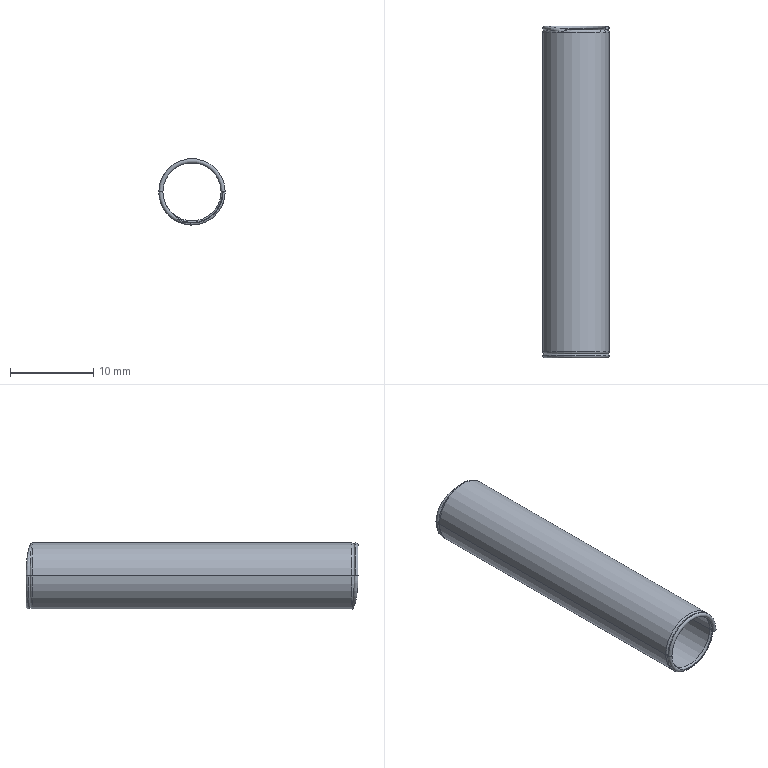Part | NX | 1 solid | 26 faces | box 8 x 40 x 8 mm | volume 464.179 mm3 | torus 18 | plane 4 | cylinder 4 | commonest cylinder face diameters 7 x2 8 x2
STEP:
#1=CARTESIAN_POINT('',(-3.75,19.5,0.));
#2=VERTEX_POINT('',#1);
#3=CARTESIAN_POINT('',(3.75,19.5,0.));
#4=VERTEX_POINT('',#3);
#5=CARTESIAN_POINT('',(0.,19.5,0.));
#6=DIRECTION('',(0.,1.,0.));
#7=DIRECTION('',(1.,0.,0.));
#8=AXIS2_PLACEMENT_3D('',#5,#6,#7);
#9=CIRCLE('',#8,3.75);
#10=EDGE_CURVE('',#2,#4,#9,.T.);
#11=ORIENTED_EDGE('',*,*,#10,.F.);
#12=CARTESIAN_POINT('',(-3.5,19.75,0.));
#13=VERTEX_POINT('',#12);
#14=CARTESIAN_POINT('',(-3.75,19.75,0.));
#15=DIRECTION('',(0.,0.,-1.));
#16=DIRECTION('',(-1.,0.,0.));
#17=AXIS2_PLACEMENT_3D('',#14,#15,#16);
#18=CIRCLE('',#17,0.25);
#19=EDGE_CURVE('',#13,#2,#18,.T.);
#20=ORIENTED_EDGE('',*,*,#19,.F.);
#21=CARTESIAN_POINT('',(-3.5,19.75,0.0215));
#22=VERTEX_POINT('',#21);
#23=CARTESIAN_POINT('',(0.,19.75,0.));
#24=DIRECTION('',(0.,-1.,0.));
#25=DIRECTION('',(-1.,0.,0.));
#26=AXIS2_PLACEMENT_3D('',#23,#24,#25);
#27=CIRCLE('',#26,3.5);
#28=EDGE_CURVE('',#22,#13,#27,.T.);
#29=ORIENTED_EDGE('',*,*,#28,.F.);
#30=CARTESIAN_POINT('',(-0.9578,19.51,3.553));
#31=VERTEX_POINT('',#30);
#32=CARTESIAN_POINT('',(-3.5,19.75,0.0215));
#33=CARTESIAN_POINT('',(-3.497,19.75,0.5366));
#34=CARTESIAN_POINT('',(-3.313,19.735,1.301));
#35=CARTESIAN_POINT('',(-2.804,19.689,2.155));
#36=CARTESIAN_POINT('',(-2.079,19.621,2.924));
#37=CARTESIAN_POINT('',(-1.377,19.557,3.326));
#38=CARTESIAN_POINT('',(-1.039,19.52,3.495));
#39=CARTESIAN_POINT('',(-0.9578,19.51,3.553));
#40=B_SPLINE_CURVE_WITH_KNOTS('',3,(#32,#33,#34,#35,#36,#37,#38,#39),.UNSPECIFIED.,.F.,.F.,(4,1,1,1,1,4),(0.,0.25,0.375,0.5,0.75,1.),.UNSPECIFIED.);
#41=EDGE_CURVE('',#31,#22,#40,.F.);
#42=ORIENTED_EDGE('',*,*,#41,.F.);
#43=CARTESIAN_POINT('',(3.68,19.51,0.));
#44=VERTEX_POINT('',#43);
#45=CARTESIAN_POINT('',(0.,19.51,0.));
#46=DIRECTION('',(0.,-1.,0.));
#47=DIRECTION('',(0.,0.,1.));
#48=AXIS2_PLACEMENT_3D('',#45,#46,#47);
#49=CIRCLE('',#48,3.68);
#50=EDGE_CURVE('',#44,#31,#49,.T.);
#51=ORIENTED_EDGE('',*,*,#50,.F.);
#52=CARTESIAN_POINT('',(3.75,19.75,0.));
#53=DIRECTION('',(0.,0.,1.));
#54=DIRECTION('',(1.,0.,0.));
#55=AXIS2_PLACEMENT_3D('',#52,#53,#54);
#56=CIRCLE('',#55,0.25);
#57=EDGE_CURVE('',#44,#4,#56,.T.);
#58=ORIENTED_EDGE('',*,*,#57,.T.);
#59=EDGE_LOOP('',(#11,#20,#29,#42,#51,#58));
#60=FACE_BOUND('',#59,.T.);
#61=CARTESIAN_POINT('',(0.,19.75,0.));
#62=DIRECTION('',(0.,-1.,0.));
#63=DIRECTION('',(-1.,0.,0.));
#64=AXIS2_PLACEMENT_3D('',#61,#62,#63);
#65=TOROIDAL_SURFACE('',#64,3.75,0.25);
#66=ADVANCED_FACE('',(#60),#65,.T.);
#67=ORIENTED_EDGE('',*,*,#50,.T.);
#68=CARTESIAN_POINT('',(-0.9704,19.51,3.622));
#69=VERTEX_POINT('',#68);
#70=CARTESIAN_POINT('',(-0.9578,19.51,3.553));
#71=CARTESIAN_POINT('',(-0.9429,19.51,3.581));
#72=CARTESIAN_POINT('',(-0.9471,19.51,3.604));
#73=CARTESIAN_POINT('',(-0.9704,19.51,3.622));
#74=B_SPLINE_CURVE_WITH_KNOTS('',3,(#70,#71,#72,#73),.UNSPECIFIED.,.F.,.F.,(4,4),(0.,1.),.UNSPECIFIED.);
#75=EDGE_CURVE('',#31,#69,#74,.T.);
#76=ORIENTED_EDGE('',*,*,#75,.T.);
#77=CARTESIAN_POINT('',(3.75,19.51,0.));
#78=VERTEX_POINT('',#77);
#79=CARTESIAN_POINT('',(0.,19.51,0.));
#80=DIRECTION('',(0.,1.,0.));
#81=DIRECTION('',(1.,0.,0.));
#82=AXIS2_PLACEMENT_3D('',#79,#80,#81);
#83=CIRCLE('',#82,3.75);
#84=EDGE_CURVE('',#69,#78,#83,.T.);
#85=ORIENTED_EDGE('',*,*,#84,.T.);
#86=CARTESIAN_POINT('',(2.812,19.51,0.));
#87=DIRECTION('',(-1.,0.,0.));
#88=VECTOR('',#87,1000.);
#89=LINE('',#86,#88);
#90=EDGE_CURVE('',#78,#44,#89,.T.);
#91=ORIENTED_EDGE('',*,*,#90,.T.);
#92=EDGE_LOOP('',(#67,#76,#85,#91));
#93=FACE_BOUND('',#92,.T.);
#94=CARTESIAN_POINT('',(1.875,19.51,0.));
#95=DIRECTION('',(0.,1.,0.));
#96=DIRECTION('',(1.,0.,0.));
#97=AXIS2_PLACEMENT_3D('',#94,#95,#96);
#98=PLANE('',#97);
#99=ADVANCED_FACE('',(#93),#98,.T.);
#100=CARTESIAN_POINT('',(-3.8,19.505,0.));
#101=VERTEX_POINT('',#100);
#102=CARTESIAN_POINT('',(-3.8,19.505,0.));
#103=CARTESIAN_POINT('',(-3.8,19.505,0.1204));
#104=CARTESIAN_POINT('',(-3.797,19.504,0.403));
#105=CARTESIAN_POINT('',(-3.736,19.496,0.9057));
#106=CARTESIAN_POINT('',(-3.632,19.485,1.311));
#107=CARTESIAN_POINT('',(-3.541,19.476,1.594));
#108=CARTESIAN_POINT('',(-3.335,19.457,2.05));
#109=CARTESIAN_POINT('',(-3.191,19.444,2.281));
#110=CARTESIAN_POINT('',(-2.929,19.422,2.652));
#111=CARTESIAN_POINT('',(-2.656,19.398,2.962));
#112=CARTESIAN_POINT('',(-2.045,19.364,3.43));
#113=CARTESIAN_POINT('',(-1.779,19.341,3.572));
#114=CARTESIAN_POINT('',(-1.267,19.4,3.777));
#115=CARTESIAN_POINT('',(-1.078,19.49,3.698));
#116=CARTESIAN_POINT('',(-1.043,19.51,3.679));
#117=CARTESIAN_POINT('',(-0.9704,19.51,3.622));
#118=B_SPLINE_CURVE_WITH_KNOTS('',3,(#102,#103,#104,#105,#106,#107,#108,#109,#110,#111,#112,#113,#114,#115,#116,#117),.UNSPECIFIED.,.F.,.F.,(4,1,1,1,1,1,1,1,1,1,1,1,1,4),(0.,0.0625,0.125,0.1562,0.1875,0.25,0.3125,0.375,0.5,0.625,0.75,0.875,0.9375,1.),.UNSPECIFIED.);
#119=EDGE_CURVE('',#69,#101,#118,.F.);
#120=ORIENTED_EDGE('',*,*,#119,.F.);
#121=ORIENTED_EDGE('',*,*,#75,.F.);
#122=ORIENTED_EDGE('',*,*,#41,.T.);
#123=ORIENTED_EDGE('',*,*,#28,.T.);
#124=CARTESIAN_POINT('',(-4.,19.75,0.));
#125=VERTEX_POINT('',#124);
#126=CARTESIAN_POINT('',(-3.75,19.75,0.));
#127=DIRECTION('',(0.,0.,-1.));
#128=DIRECTION('',(-1.,0.,0.));
#129=AXIS2_PLACEMENT_3D('',#126,#127,#128);
#130=CIRCLE('',#129,0.25);
#131=EDGE_CURVE('',#125,#13,#130,.T.);
#132=ORIENTED_EDGE('',*,*,#131,.F.);
#133=CARTESIAN_POINT('',(-3.75,19.75,0.));
#134=DIRECTION('',(0.,0.,-1.));
#135=DIRECTION('',(-1.,0.,0.));
#136=AXIS2_PLACEMENT_3D('',#133,#134,#135);
#137=CIRCLE('',#136,0.25);
#138=EDGE_CURVE('',#101,#125,#137,.T.);
#139=ORIENTED_EDGE('',*,*,#138,.F.);
#140=EDGE_LOOP('',(#120,#121,#122,#123,#132,#139));
#141=FACE_BOUND('',#140,.T.);
#142=CARTESIAN_POINT('',(-0.1131,19.109,0.));
#143=DIRECTION('',(-0.1736,-0.9848,0.));
#144=DIRECTION('',(-0.9848,0.1736,0.));
#145=AXIS2_PLACEMENT_3D('',#142,#143,#144);
#146=TOROIDAL_SURFACE('',#145,3.693,0.25);
#147=ADVANCED_FACE('',(#141),#146,.T.);
#148=CARTESIAN_POINT('',(3.68,-19.51,0.));
#149=VERTEX_POINT('',#148);
#150=CARTESIAN_POINT('',(-0.9578,-19.51,-3.553));
#151=VERTEX_POINT('',#150);
#152=CARTESIAN_POINT('',(0.,-19.51,0.));
#153=DIRECTION('',(0.,1.,0.));
#154=DIRECTION('',(0.,0.,1.));
#155=AXIS2_PLACEMENT_3D('',#152,#153,#154);
#156=CIRCLE('',#155,3.68);
#157=EDGE_CURVE('',#149,#151,#156,.T.);
#158=ORIENTED_EDGE('',*,*,#157,.T.);
#159=CARTESIAN_POINT('',(-0.9704,-19.51,-3.622));
#160=VERTEX_POINT('',#159);
#161=CARTESIAN_POINT('',(-0.9578,-19.51,-3.553));
#162=CARTESIAN_POINT('',(-0.9429,-19.51,-3.581));
#163=CARTESIAN_POINT('',(-0.9471,-19.51,-3.604));
#164=CARTESIAN_POINT('',(-0.9704,-19.51,-3.622));
#165=B_SPLINE_CURVE_WITH_KNOTS('',3,(#161,#162,#163,#164),.UNSPECIFIED.,.F.,.F.,(4,4),(0.,1.),.UNSPECIFIED.);
#166=EDGE_CURVE('',#151,#160,#165,.T.);
#167=ORIENTED_EDGE('',*,*,#166,.T.);
#168=CARTESIAN_POINT('',(3.75,-19.51,0.));
#169=VERTEX_POINT('',#168);
#170=CARTESIAN_POINT('',(0.,-19.51,0.));
#171=DIRECTION('',(0.,1.,0.));
#172=DIRECTION('',(1.,0.,0.));
#173=AXIS2_PLACEMENT_3D('',#170,#171,#172);
#174=CIRCLE('',#173,3.75);
#175=EDGE_CURVE('',#169,#160,#174,.T.);
#176=ORIENTED_EDGE('',*,*,#175,.F.);
#177=CARTESIAN_POINT('',(2.812,-19.51,0.));
#178=DIRECTION('',(-1.,0.,0.));
#179=VECTOR('',#178,1000.);
#180=LINE('',#177,#179);
#181=EDGE_CURVE('',#169,#149,#180,.T.);
#182=ORIENTED_EDGE('',*,*,#181,.T.);
#183=EDGE_LOOP('',(#158,#167,#176,#182));
#184=FACE_BOUND('',#183,.T.);
#185=CARTESIAN_POINT('',(1.875,-19.51,0.));
#186=DIRECTION('',(0.,-1.,0.));
#187=DIRECTION('',(0.,0.,-1.));
#188=AXIS2_PLACEMENT_3D('',#185,#186,#187);
#189=PLANE('',#188);
#190=ADVANCED_FACE('',(#184),#189,.T.);
#191=ORIENTED_EDGE('',*,*,#10,.T.);
#192=CARTESIAN_POINT('',(3.5,19.25,0.));
#193=VERTEX_POINT('',#192);
#194=CARTESIAN_POINT('',(3.75,19.25,0.));
#195=DIRECTION('',(0.,0.,-1.));
#196=DIRECTION('',(-1.,0.,0.));
#197=AXIS2_PLACEMENT_3D('',#194,#195,#196);
#198=CIRCLE('',#197,0.25);
#199=EDGE_CURVE('',#193,#4,#198,.T.);
#200=ORIENTED_EDGE('',*,*,#199,.F.);
#201=CARTESIAN_POINT('',(-3.5,19.25,0.));
#202=VERTEX_POINT('',#201);
#203=CARTESIAN_POINT('',(0.,19.25,0.));
#204=DIRECTION('',(0.,1.,0.));
#205=DIRECTION('',(1.,0.,0.));
#206=AXIS2_PLACEMENT_3D('',#203,#204,#205);
#207=CIRCLE('',#206,3.5);
#208=EDGE_CURVE('',#202,#193,#207,.T.);
#209=ORIENTED_EDGE('',*,*,#208,.F.);
#210=CARTESIAN_POINT('',(-3.75,19.25,0.));
#211=DIRECTION('',(0.,0.,1.));
#212=DIRECTION('',(1.,0.,0.));
#213=AXIS2_PLACEMENT_3D('',#210,#211,#212);
#214=CIRCLE('',#213,0.25);
#215=EDGE_CURVE('',#202,#2,#214,.T.);
#216=ORIENTED_EDGE('',*,*,#215,.T.);
#217=EDGE_LOOP('',(#191,#200,#209,#216));
#218=FACE_BOUND('',#217,.T.);
#219=CARTESIAN_POINT('',(0.,19.25,0.));
#220=DIRECTION('',(0.,1.,0.));
#221=DIRECTION('',(1.,0.,0.));
#222=AXIS2_PLACEMENT_3D('',#219,#220,#221);
#223=TOROIDAL_SURFACE('',#222,3.75,0.25);
#224=ADVANCED_FACE('',(#218),#223,.T.);
#225=CARTESIAN_POINT('',(-4.,-19.75,0.));
#226=VERTEX_POINT('',#225);
#227=CARTESIAN_POINT('',(-3.8,-19.505,0.));
#228=VERTEX_POINT('',#227);
#229=CARTESIAN_POINT('',(-3.75,-19.75,0.));
#230=DIRECTION('',(0.,0.,-1.));
#231=DIRECTION('',(-1.,0.,0.));
#232=AXIS2_PLACEMENT_3D('',#229,#230,#231);
#233=CIRCLE('',#232,0.25);
#234=EDGE_CURVE('',#226,#228,#233,.T.);
#235=ORIENTED_EDGE('',*,*,#234,.T.);
#236=CARTESIAN_POINT('',(-3.8,-19.505,0.));
#237=CARTESIAN_POINT('',(-3.8,-19.505,-0.1568));
#238=CARTESIAN_POINT('',(-3.794,-19.504,-0.4603));
#239=CARTESIAN_POINT('',(-3.721,-19.495,-0.9752));
#240=CARTESIAN_POINT('',(-3.549,-19.477,-1.621));
#241=CARTESIAN_POINT('',(-3.279,-19.452,-2.163));
#242=CARTESIAN_POINT('',(-2.911,-19.419,-2.695));
#243=CARTESIAN_POINT('',(-2.445,-19.384,-3.138));
#244=CARTESIAN_POINT('',(-2.135,-19.367,-3.356));
#245=CARTESIAN_POINT('',(-1.981,-19.359,-3.456));
#246=CARTESIAN_POINT('',(-1.669,-19.356,-3.619));
#247=CARTESIAN_POINT('',(-1.519,-19.361,-3.673));
#248=CARTESIAN_POINT('',(-1.282,-19.404,-3.765));
#249=CARTESIAN_POINT('',(-1.07,-19.492,-3.698));
#250=CARTESIAN_POINT('',(-1.042,-19.51,-3.678));
#251=CARTESIAN_POINT('',(-0.9704,-19.51,-3.622));
#252=B_SPLINE_CURVE_WITH_KNOTS('',3,(#236,#237,#238,#239,#240,#241,#242,#243,#244,#245,#246,#247,#248,#249,#250,#251),.UNSPECIFIED.,.F.,.F.,(4,1,1,1,1,1,1,1,1,1,1,1,1,4),(0.,0.125,0.1875,0.25,0.375,0.5,0.625,0.6875,0.75,0.8125,0.875,0.9375,0.9688,1.),.UNSPECIFIED.);
#253=EDGE_CURVE('',#160,#228,#252,.F.);
#254=ORIENTED_EDGE('',*,*,#253,.F.);
#255=ORIENTED_EDGE('',*,*,#166,.F.);
#256=CARTESIAN_POINT('',(-3.5,-19.75,-0.0215));
#257=VERTEX_POINT('',#256);
#258=CARTESIAN_POINT('',(-0.9578,-19.51,-3.553));
#259=CARTESIAN_POINT('',(-1.039,-19.52,-3.495));
#260=CARTESIAN_POINT('',(-1.302,-19.548,-3.374));
#261=CARTESIAN_POINT('',(-1.834,-19.599,-3.049));
#262=CARTESIAN_POINT('',(-2.247,-19.637,-2.744));
#263=CARTESIAN_POINT('',(-2.804,-19.687,-2.155));
#264=CARTESIAN_POINT('',(-3.311,-19.732,-1.305));
#265=CARTESIAN_POINT('',(-3.497,-19.75,-0.5384));
#266=CARTESIAN_POINT('',(-3.5,-19.75,-0.0215));
#267=B_SPLINE_CURVE_WITH_KNOTS('',3,(#258,#259,#260,#261,#262,#263,#264,#265,#266),.UNSPECIFIED.,.F.,.F.,(4,1,1,1,1,1,4),(0.,0.25,0.375,0.5,0.625,0.75,1.),.UNSPECIFIED.);
#268=EDGE_CURVE('',#257,#151,#267,.F.);
#269=ORIENTED_EDGE('',*,*,#268,.F.);
#270=CARTESIAN_POINT('',(-3.5,-19.75,0.));
#271=VERTEX_POINT('',#270);
#272=CARTESIAN_POINT('',(0.,-19.75,0.));
#273=DIRECTION('',(0.,-1.,0.));
#274=DIRECTION('',(-1.,0.,0.));
#275=AXIS2_PLACEMENT_3D('',#272,#273,#274);
#276=CIRCLE('',#275,3.5);
#277=EDGE_CURVE('',#257,#271,#276,.F.);
#278=ORIENTED_EDGE('',*,*,#277,.T.);
#279=CARTESIAN_POINT('',(-3.75,-19.75,0.));
#280=DIRECTION('',(0.,0.,-1.));
#281=DIRECTION('',(-1.,0.,0.));
#282=AXIS2_PLACEMENT_3D('',#279,#280,#281);
#283=CIRCLE('',#282,0.25);
#284=EDGE_CURVE('',#271,#226,#283,.T.);
#285=ORIENTED_EDGE('',*,*,#284,.T.);
#286=EDGE_LOOP('',(#235,#254,#255,#269,#278,#285));
#287=FACE_BOUND('',#286,.T.);
#288=CARTESIAN_POINT('',(-0.1131,-19.109,0.));
#289=DIRECTION('',(0.1736,-0.9848,0.));
#290=DIRECTION('',(-0.9848,-0.1736,0.));
#291=AXIS2_PLACEMENT_3D('',#288,#289,#290);
#292=TOROIDAL_SURFACE('',#291,3.693,0.25);
#293=ADVANCED_FACE('',(#287),#292,.T.);
#294=CARTESIAN_POINT('',(3.8,19.505,0.));
#295=VERTEX_POINT('',#294);
#296=CARTESIAN_POINT('',(3.75,19.26,0.));
#297=DIRECTION('',(0.,0.,-1.));
#298=DIRECTION('',(-1.,0.,0.));
#299=AXIS2_PLACEMENT_3D('',#296,#297,#298);
#300=CIRCLE('',#299,0.25);
#301=EDGE_CURVE('',#78,#295,#300,.T.);
#302=ORIENTED_EDGE('',*,*,#301,.T.);
#303=CARTESIAN_POINT('',(4.,19.75,0.));
#304=VERTEX_POINT('',#303);
#305=CARTESIAN_POINT('',(3.75,19.75,0.));
#306=DIRECTION('',(0.,0.,1.));
#307=DIRECTION('',(1.,0.,0.));
#308=AXIS2_PLACEMENT_3D('',#305,#306,#307);
#309=CIRCLE('',#308,0.25);
#310=EDGE_CURVE('',#295,#304,#309,.T.);
#311=ORIENTED_EDGE('',*,*,#310,.T.);
#312=CARTESIAN_POINT('',(3.5,19.75,0.));
#313=VERTEX_POINT('',#312);
#314=CARTESIAN_POINT('',(3.75,19.75,0.));
#315=DIRECTION('',(0.,0.,1.));
#316=DIRECTION('',(1.,0.,0.));
#317=AXIS2_PLACEMENT_3D('',#314,#315,#316);
#318=CIRCLE('',#317,0.25);
#319=EDGE_CURVE('',#304,#313,#318,.T.);
#320=ORIENTED_EDGE('',*,*,#319,.T.);
#321=CARTESIAN_POINT('',(3.75,19.75,0.));
#322=DIRECTION('',(0.,0.,1.));
#323=DIRECTION('',(1.,0.,0.));
#324=AXIS2_PLACEMENT_3D('',#321,#322,#323);
#325=CIRCLE('',#324,0.25);
#326=EDGE_CURVE('',#313,#44,#325,.T.);
#327=ORIENTED_EDGE('',*,*,#326,.T.);
#328=ORIENTED_EDGE('',*,*,#90,.F.);
#329=EDGE_LOOP('',(#302,#311,#320,#327,#328));
#330=FACE_BOUND('',#329,.T.);
#331=CARTESIAN_POINT('',(3.75,19.75,0.));
#332=DIRECTION('',(0.,0.,-1.));
#333=DIRECTION('',(-1.,0.,0.));
#334=AXIS2_PLACEMENT_3D('',#331,#332,#333);
#335=PLANE('',#334);
#336=ADVANCED_FACE('',(#330),#335,.F.);
#337=CARTESIAN_POINT('',(-3.75,-19.5,0.));
#338=VERTEX_POINT('',#337);
#339=CARTESIAN_POINT('',(3.75,-19.5,0.));
#340=VERTEX_POINT('',#339);
#341=CARTESIAN_POINT('',(0.,-19.5,0.));
#342=DIRECTION('',(0.,1.,0.));
#343=DIRECTION('',(1.,0.,0.));
#344=AXIS2_PLACEMENT_3D('',#341,#342,#343);
#345=CIRCLE('',#344,3.75);
#346=EDGE_CURVE('',#338,#340,#345,.T.);
#347=ORIENTED_EDGE('',*,*,#346,.T.);
#348=CARTESIAN_POINT('',(3.75,-19.75,0.));
#349=DIRECTION('',(0.,0.,1.));
#350=DIRECTION('',(1.,0.,0.));
#351=AXIS2_PLACEMENT_3D('',#348,#349,#350);
#352=CIRCLE('',#351,0.25);
#353=EDGE_CURVE('',#149,#340,#352,.F.);
#354=ORIENTED_EDGE('',*,*,#353,.F.);
#355=CARTESIAN_POINT('',(3.5,-19.75,0.));
#356=VERTEX_POINT('',#355);
#357=CARTESIAN_POINT('',(3.75,-19.75,0.));
#358=DIRECTION('',(0.,0.,1.));
#359=DIRECTION('',(1.,0.,0.));
#360=AXIS2_PLACEMENT_3D('',#357,#358,#359);
#361=CIRCLE('',#360,0.25);
#362=EDGE_CURVE('',#149,#356,#361,.T.);
#363=ORIENTED_EDGE('',*,*,#362,.T.);
#364=CARTESIAN_POINT('',(0.,-19.75,0.));
#365=DIRECTION('',(0.,-1.,0.));
#366=DIRECTION('',(-1.,0.,0.));
#367=AXIS2_PLACEMENT_3D('',#364,#365,#366);
#368=CIRCLE('',#367,3.5);
#369=EDGE_CURVE('',#356,#271,#368,.T.);
#370=ORIENTED_EDGE('',*,*,#369,.T.);
#371=CARTESIAN_POINT('',(-3.75,-19.75,0.));
#372=DIRECTION('',(0.,0.,-1.));
#373=DIRECTION('',(-1.,0.,0.));
#374=AXIS2_PLACEMENT_3D('',#371,#372,#373);
#375=CIRCLE('',#374,0.25);
#376=EDGE_CURVE('',#271,#338,#375,.F.);
#377=ORIENTED_EDGE('',*,*,#376,.T.);
#378=EDGE_LOOP('',(#347,#354,#363,#370,#377));
#379=FACE_BOUND('',#378,.T.);
#380=CARTESIAN_POINT('',(0.,-19.75,0.));
#381=DIRECTION('',(0.,-1.,0.));
#382=DIRECTION('',(-1.,0.,0.));
#383=AXIS2_PLACEMENT_3D('',#380,#381,#382);
#384=TOROIDAL_SURFACE('',#383,3.75,0.25);
#385=ADVANCED_FACE('',(#379),#384,.T.);
#386=CARTESIAN_POINT('',(-4.,-19.26,0.));
#387=VERTEX_POINT('',#386);
#388=CARTESIAN_POINT('',(4.,-19.26,0.));
#389=VERTEX_POINT('',#388);
#390=CARTESIAN_POINT('',(0.,-19.26,0.));
#391=DIRECTION('',(0.,1.,0.));
#392=DIRECTION('',(1.,0.,0.));
#393=AXIS2_PLACEMENT_3D('',#390,#391,#392);
#394=CIRCLE('',#393,4.);
#395=EDGE_CURVE('',#387,#389,#394,.T.);
#396=ORIENTED_EDGE('',*,*,#395,.F.);
#397=CARTESIAN_POINT('',(-3.75,-19.26,0.));
#398=DIRECTION('',(0.,0.,1.));
#399=DIRECTION('',(1.,0.,0.));
#400=AXIS2_PLACEMENT_3D('',#397,#398,#399);
#401=CIRCLE('',#400,0.25);
#402=EDGE_CURVE('',#228,#387,#401,.F.);
#403=ORIENTED_EDGE('',*,*,#402,.F.);
#404=CARTESIAN_POINT('',(3.8,-19.505,0.));
#405=VERTEX_POINT('',#404);
#406=CARTESIAN_POINT('',(0.,-19.505,0.));
#407=DIRECTION('',(0.,1.,0.));
#408=DIRECTION('',(0.,0.,-1.));
#409=AXIS2_PLACEMENT_3D('',#406,#407,#408);
#410=CIRCLE('',#409,3.8);
#411=EDGE_CURVE('',#228,#405,#410,.T.);
#412=ORIENTED_EDGE('',*,*,#411,.T.);
#413=CARTESIAN_POINT('',(3.75,-19.26,0.));
#414=DIRECTION('',(0.,0.,-1.));
#415=DIRECTION('',(-1.,0.,0.));
#416=AXIS2_PLACEMENT_3D('',#413,#414,#415);
#417=CIRCLE('',#416,0.25);
#418=EDGE_CURVE('',#405,#389,#417,.F.);
#419=ORIENTED_EDGE('',*,*,#418,.T.);
#420=EDGE_LOOP('',(#396,#403,#412,#419));
#421=FACE_BOUND('',#420,.T.);
#422=CARTESIAN_POINT('',(0.,-19.26,0.));
#423=DIRECTION('',(0.,1.,0.));
#424=DIRECTION('',(1.,0.,0.));
#425=AXIS2_PLACEMENT_3D('',#422,#423,#424);
#426=TOROIDAL_SURFACE('',#425,3.75,0.25);
#427=ADVANCED_FACE('',(#421),#426,.T.);
#428=CARTESIAN_POINT('',(-3.5,-19.25,0.));
#429=VERTEX_POINT('',#428);
#430=CARTESIAN_POINT('',(3.5,-19.25,0.));
#431=VERTEX_POINT('',#430);
#432=CARTESIAN_POINT('',(0.,-19.25,0.));
#433=DIRECTION('',(0.,1.,0.));
#434=DIRECTION('',(1.,0.,0.));
#435=AXIS2_PLACEMENT_3D('',#432,#433,#434);
#436=CIRCLE('',#435,3.5);
#437=EDGE_CURVE('',#429,#431,#436,.T.);
#438=ORIENTED_EDGE('',*,*,#437,.F.);
#439=CARTESIAN_POINT('',(-3.5,0.,0.));
#440=DIRECTION('',(0.,-1.,0.));
#441=VECTOR('',#440,1000.);
#442=LINE('',#439,#441);
#443=EDGE_CURVE('',#202,#429,#442,.T.);
#444=ORIENTED_EDGE('',*,*,#443,.F.);
#445=ORIENTED_EDGE('',*,*,#208,.T.);
#446=CARTESIAN_POINT('',(3.5,0.,0.));
#447=DIRECTION('',(0.,-1.,0.));
#448=VECTOR('',#447,1000.);
#449=LINE('',#446,#448);
#450=EDGE_CURVE('',#193,#431,#449,.T.);
#451=ORIENTED_EDGE('',*,*,#450,.T.);
#452=EDGE_LOOP('',(#438,#444,#445,#451));
#453=FACE_BOUND('',#452,.T.);
#454=CARTESIAN_POINT('',(0.,0.,0.));
#455=DIRECTION('',(0.,-1.,0.));
#456=DIRECTION('',(1.,0.,0.));
#457=AXIS2_PLACEMENT_3D('',#454,#455,#456);
#458=CYLINDRICAL_SURFACE('',#457,3.5);
#459=ADVANCED_FACE('',(#453),#458,.F.);
#460=CARTESIAN_POINT('',(-4.,19.26,0.));
#461=VERTEX_POINT('',#460);
#462=CARTESIAN_POINT('',(4.,19.26,0.));
#463=VERTEX_POINT('',#462);
#464=CARTESIAN_POINT('',(0.,19.26,0.));
#465=DIRECTION('',(0.,1.,0.));
#466=DIRECTION('',(1.,0.,0.));
#467=AXIS2_PLACEMENT_3D('',#464,#465,#466);
#468=CIRCLE('',#467,4.);
#469=EDGE_CURVE('',#461,#463,#468,.T.);
#470=ORIENTED_EDGE('',*,*,#469,.F.);
#471=CARTESIAN_POINT('',(-4.,0.,0.));
#472=DIRECTION('',(0.,-1.,0.));
#473=VECTOR('',#472,1000.);
#474=LINE('',#471,#473);
#475=EDGE_CURVE('',#461,#387,#474,.T.);
#476=ORIENTED_EDGE('',*,*,#475,.T.);
#477=ORIENTED_EDGE('',*,*,#395,.T.);
#478=CARTESIAN_POINT('',(4.,0.,0.));
#479=DIRECTION('',(0.,-1.,0.));
#480=VECTOR('',#479,1000.);
#481=LINE('',#478,#480);
#482=EDGE_CURVE('',#463,#389,#481,.T.);
#483=ORIENTED_EDGE('',*,*,#482,.F.);
#484=EDGE_LOOP('',(#470,#476,#477,#483));
#485=FACE_BOUND('',#484,.T.);
#486=CARTESIAN_POINT('',(0.,0.,0.));
#487=DIRECTION('',(0.,-1.,0.));
#488=DIRECTION('',(1.,0.,0.));
#489=AXIS2_PLACEMENT_3D('',#486,#487,#488);
#490=CYLINDRICAL_SURFACE('',#489,4.);
#491=ADVANCED_FACE('',(#485),#490,.T.);
#492=ORIENTED_EDGE('',*,*,#181,.F.);
#493=CARTESIAN_POINT('',(3.75,-19.26,0.));
#494=DIRECTION('',(0.,0.,-1.));
#495=DIRECTION('',(-1.,0.,0.));
#496=AXIS2_PLACEMENT_3D('',#493,#494,#495);
#497=CIRCLE('',#496,0.25);
#498=EDGE_CURVE('',#405,#169,#497,.T.);
#499=ORIENTED_EDGE('',*,*,#498,.F.);
#500=CARTESIAN_POINT('',(4.,-19.75,0.));
#501=VERTEX_POINT('',#500);
#502=CARTESIAN_POINT('',(3.75,-19.75,0.));
#503=DIRECTION('',(0.,0.,1.));
#504=DIRECTION('',(1.,0.,0.));
#505=AXIS2_PLACEMENT_3D('',#502,#503,#504);
#506=CIRCLE('',#505,0.25);
#507=EDGE_CURVE('',#501,#405,#506,.T.);
#508=ORIENTED_EDGE('',*,*,#507,.F.);
#509=CARTESIAN_POINT('',(3.75,-19.75,0.));
#510=DIRECTION('',(0.,0.,1.));
#511=DIRECTION('',(1.,0.,0.));
#512=AXIS2_PLACEMENT_3D('',#509,#510,#511);
#513=CIRCLE('',#512,0.25);
#514=EDGE_CURVE('',#356,#501,#513,.T.);
#515=ORIENTED_EDGE('',*,*,#514,.F.);
#516=ORIENTED_EDGE('',*,*,#362,.F.);
#517=EDGE_LOOP('',(#492,#499,#508,#515,#516));
#518=FACE_BOUND('',#517,.T.);
#519=CARTESIAN_POINT('',(3.75,-19.75,0.));
#520=DIRECTION('',(0.,0.,-1.));
#521=DIRECTION('',(0.,-1.,0.));
#522=AXIS2_PLACEMENT_3D('',#519,#520,#521);
#523=PLANE('',#522);
#524=ADVANCED_FACE('',(#518),#523,.T.);
#525=ORIENTED_EDGE('',*,*,#119,.T.);
#526=CARTESIAN_POINT('',(-3.75,19.26,0.));
#527=DIRECTION('',(0.,0.,1.));
#528=DIRECTION('',(1.,0.,0.));
#529=AXIS2_PLACEMENT_3D('',#526,#527,#528);
#530=CIRCLE('',#529,0.25);
#531=EDGE_CURVE('',#101,#461,#530,.T.);
#532=ORIENTED_EDGE('',*,*,#531,.T.);
#533=ORIENTED_EDGE('',*,*,#469,.T.);
#534=CARTESIAN_POINT('',(3.75,19.26,0.));
#535=DIRECTION('',(0.,0.,-1.));
#536=DIRECTION('',(-1.,0.,0.));
#537=AXIS2_PLACEMENT_3D('',#534,#535,#536);
#538=CIRCLE('',#537,0.25);
#539=EDGE_CURVE('',#295,#463,#538,.T.);
#540=ORIENTED_EDGE('',*,*,#539,.F.);
#541=ORIENTED_EDGE('',*,*,#301,.F.);
#542=ORIENTED_EDGE('',*,*,#84,.F.);
#543=EDGE_LOOP('',(#525,#532,#533,#540,#541,#542));
#544=FACE_BOUND('',#543,.T.);
#545=CARTESIAN_POINT('',(0.,19.26,0.));
#546=DIRECTION('',(0.,1.,0.));
#547=DIRECTION('',(1.,0.,0.));
#548=AXIS2_PLACEMENT_3D('',#545,#546,#547);
#549=TOROIDAL_SURFACE('',#548,3.75,0.25);
#550=ADVANCED_FACE('',(#544),#549,.T.);
#551=ORIENTED_EDGE('',*,*,#346,.F.);
#552=CARTESIAN_POINT('',(-3.75,-19.25,0.));
#553=DIRECTION('',(0.,0.,1.));
#554=DIRECTION('',(1.,0.,0.));
#555=AXIS2_PLACEMENT_3D('',#552,#553,#554);
#556=CIRCLE('',#555,0.25);
#557=EDGE_CURVE('',#338,#429,#556,.T.);
#558=ORIENTED_EDGE('',*,*,#557,.T.);
#559=ORIENTED_EDGE('',*,*,#437,.T.);
#560=CARTESIAN_POINT('',(3.75,-19.25,0.));
#561=DIRECTION('',(0.,0.,-1.));
#562=DIRECTION('',(-1.,0.,0.));
#563=AXIS2_PLACEMENT_3D('',#560,#561,#562);
#564=CIRCLE('',#563,0.25);
#565=EDGE_CURVE('',#340,#431,#564,.T.);
#566=ORIENTED_EDGE('',*,*,#565,.F.);
#567=EDGE_LOOP('',(#551,#558,#559,#566));
#568=FACE_BOUND('',#567,.T.);
#569=CARTESIAN_POINT('',(0.,-19.25,0.));
#570=DIRECTION('',(0.,1.,0.));
#571=DIRECTION('',(1.,0.,0.));
#572=AXIS2_PLACEMENT_3D('',#569,#570,#571);
#573=TOROIDAL_SURFACE('',#572,3.75,0.25);
#574=ADVANCED_FACE('',(#568),#573,.T.);
#575=ORIENTED_EDGE('',*,*,#482,.T.);
#576=CARTESIAN_POINT('',(0.,-19.26,0.));
#577=DIRECTION('',(0.,1.,0.));
#578=DIRECTION('',(1.,0.,0.));
#579=AXIS2_PLACEMENT_3D('',#576,#577,#578);
#580=CIRCLE('',#579,4.);
#581=EDGE_CURVE('',#389,#387,#580,.T.);
#582=ORIENTED_EDGE('',*,*,#581,.T.);
#583=ORIENTED_EDGE('',*,*,#475,.F.);
#584=CARTESIAN_POINT('',(0.,19.26,0.));
#585=DIRECTION('',(0.,1.,0.));
#586=DIRECTION('',(1.,0.,0.));
#587=AXIS2_PLACEMENT_3D('',#584,#585,#586);
#588=CIRCLE('',#587,4.);
#589=EDGE_CURVE('',#463,#461,#588,.T.);
#590=ORIENTED_EDGE('',*,*,#589,.F.);
#591=EDGE_LOOP('',(#575,#582,#583,#590));
#592=FACE_BOUND('',#591,.T.);
#593=CARTESIAN_POINT('',(0.,0.,0.));
#594=DIRECTION('',(0.,-1.,0.));
#595=DIRECTION('',(1.,0.,0.));
#596=AXIS2_PLACEMENT_3D('',#593,#594,#595);
#597=CYLINDRICAL_SURFACE('',#596,4.);
#598=ADVANCED_FACE('',(#592),#597,.T.);
#599=CARTESIAN_POINT('',(0.,19.75,0.));
#600=DIRECTION('',(0.,-1.,0.));
#601=DIRECTION('',(-1.,0.,0.));
#602=AXIS2_PLACEMENT_3D('',#599,#600,#601);
#603=CIRCLE('',#602,4.);
#604=EDGE_CURVE('',#125,#304,#603,.T.);
#605=ORIENTED_EDGE('',*,*,#604,.F.);
#606=ORIENTED_EDGE('',*,*,#131,.T.);
#607=CARTESIAN_POINT('',(0.,19.75,0.));
#608=DIRECTION('',(0.,-1.,0.));
#609=DIRECTION('',(-1.,0.,0.));
#610=AXIS2_PLACEMENT_3D('',#607,#608,#609);
#611=CIRCLE('',#610,3.5);
#612=EDGE_CURVE('',#13,#313,#611,.T.);
#613=ORIENTED_EDGE('',*,*,#612,.T.);
#614=ORIENTED_EDGE('',*,*,#319,.F.);
#615=EDGE_LOOP('',(#605,#606,#613,#614));
#616=FACE_BOUND('',#615,.T.);
#617=CARTESIAN_POINT('',(0.,19.75,0.));
#618=DIRECTION('',(0.,-1.,0.));
#619=DIRECTION('',(-1.,0.,0.));
#620=AXIS2_PLACEMENT_3D('',#617,#618,#619);
#621=TOROIDAL_SURFACE('',#620,3.75,0.25);
#622=ADVANCED_FACE('',(#616),#621,.T.);
#623=ORIENTED_EDGE('',*,*,#604,.T.);
#624=ORIENTED_EDGE('',*,*,#310,.F.);
#625=CARTESIAN_POINT('',(0.,19.505,0.));
#626=DIRECTION('',(0.,-1.,0.));
#627=DIRECTION('',(0.,0.,-1.));
#628=AXIS2_PLACEMENT_3D('',#625,#626,#627);
#629=CIRCLE('',#628,3.8);
#630=EDGE_CURVE('',#101,#295,#629,.T.);
#631=ORIENTED_EDGE('',*,*,#630,.F.);
#632=ORIENTED_EDGE('',*,*,#138,.T.);
#633=EDGE_LOOP('',(#623,#624,#631,#632));
#634=FACE_BOUND('',#633,.T.);
#635=CARTESIAN_POINT('',(0.,19.75,0.));
#636=DIRECTION('',(0.,-1.,0.));
#637=DIRECTION('',(-1.,0.,0.));
#638=AXIS2_PLACEMENT_3D('',#635,#636,#637);
#639=TOROIDAL_SURFACE('',#638,3.75,0.25);
#640=ADVANCED_FACE('',(#634),#639,.T.);
#641=CARTESIAN_POINT('',(0.,-19.75,0.));
#642=DIRECTION('',(0.,-1.,0.));
#643=DIRECTION('',(-1.,0.,0.));
#644=AXIS2_PLACEMENT_3D('',#641,#642,#643);
#645=CIRCLE('',#644,4.);
#646=EDGE_CURVE('',#501,#226,#645,.T.);
#647=ORIENTED_EDGE('',*,*,#646,.T.);
#648=ORIENTED_EDGE('',*,*,#284,.F.);
#649=ORIENTED_EDGE('',*,*,#369,.F.);
#650=ORIENTED_EDGE('',*,*,#514,.T.);
#651=EDGE_LOOP('',(#647,#648,#649,#650));
#652=FACE_BOUND('',#651,.T.);
#653=CARTESIAN_POINT('',(0.,-19.75,0.));
#654=DIRECTION('',(0.,-1.,0.));
#655=DIRECTION('',(-1.,0.,0.));
#656=AXIS2_PLACEMENT_3D('',#653,#654,#655);
#657=TOROIDAL_SURFACE('',#656,3.75,0.25);
#658=ADVANCED_FACE('',(#652),#657,.T.);
#659=ORIENTED_EDGE('',*,*,#507,.T.);
#660=ORIENTED_EDGE('',*,*,#411,.F.);
#661=ORIENTED_EDGE('',*,*,#234,.F.);
#662=ORIENTED_EDGE('',*,*,#646,.F.);
#663=EDGE_LOOP('',(#659,#660,#661,#662));
#664=FACE_BOUND('',#663,.T.);
#665=CARTESIAN_POINT('',(0.,-19.75,0.));
#666=DIRECTION('',(0.,-1.,0.));
#667=DIRECTION('',(-1.,0.,0.));
#668=AXIS2_PLACEMENT_3D('',#665,#666,#667);
#669=TOROIDAL_SURFACE('',#668,3.75,0.25);
#670=ADVANCED_FACE('',(#664),#669,.T.);
#671=ORIENTED_EDGE('',*,*,#450,.F.);
#672=CARTESIAN_POINT('',(0.,19.25,0.));
#673=DIRECTION('',(0.,1.,0.));
#674=DIRECTION('',(1.,0.,0.));
#675=AXIS2_PLACEMENT_3D('',#672,#673,#674);
#676=CIRCLE('',#675,3.5);
#677=EDGE_CURVE('',#193,#202,#676,.T.);
#678=ORIENTED_EDGE('',*,*,#677,.T.);
#679=ORIENTED_EDGE('',*,*,#443,.T.);
#680=CARTESIAN_POINT('',(0.,-19.25,0.));
#681=DIRECTION('',(0.,1.,0.));
#682=DIRECTION('',(1.,0.,0.));
#683=AXIS2_PLACEMENT_3D('',#680,#681,#682);
#684=CIRCLE('',#683,3.5);
#685=EDGE_CURVE('',#431,#429,#684,.T.);
#686=ORIENTED_EDGE('',*,*,#685,.F.);
#687=EDGE_LOOP('',(#671,#678,#679,#686));
#688=FACE_BOUND('',#687,.T.);
#689=CARTESIAN_POINT('',(0.,0.,0.));
#690=DIRECTION('',(0.,-1.,0.));
#691=DIRECTION('',(1.,0.,0.));
#692=AXIS2_PLACEMENT_3D('',#689,#690,#691);
#693=CYLINDRICAL_SURFACE('',#692,3.5);
#694=ADVANCED_FACE('',(#688),#693,.F.);
#695=ORIENTED_EDGE('',*,*,#498,.T.);
#696=ORIENTED_EDGE('',*,*,#175,.T.);
#697=ORIENTED_EDGE('',*,*,#253,.T.);
#698=ORIENTED_EDGE('',*,*,#402,.T.);
#699=ORIENTED_EDGE('',*,*,#581,.F.);
#700=ORIENTED_EDGE('',*,*,#418,.F.);
#701=EDGE_LOOP('',(#695,#696,#697,#698,#699,#700));
#702=FACE_BOUND('',#701,.T.);
#703=CARTESIAN_POINT('',(0.,-19.26,0.));
#704=DIRECTION('',(0.,1.,0.));
#705=DIRECTION('',(1.,0.,0.));
#706=AXIS2_PLACEMENT_3D('',#703,#704,#705);
#707=TOROIDAL_SURFACE('',#706,3.75,0.25);
#708=ADVANCED_FACE('',(#702),#707,.T.);
#709=ORIENTED_EDGE('',*,*,#565,.T.);
#710=ORIENTED_EDGE('',*,*,#685,.T.);
#711=ORIENTED_EDGE('',*,*,#557,.F.);
#712=CARTESIAN_POINT('',(0.,-19.5,0.));
#713=DIRECTION('',(0.,1.,0.));
#714=DIRECTION('',(1.,0.,0.));
#715=AXIS2_PLACEMENT_3D('',#712,#713,#714);
#716=CIRCLE('',#715,3.75);
#717=EDGE_CURVE('',#340,#338,#716,.T.);
#718=ORIENTED_EDGE('',*,*,#717,.F.);
#719=EDGE_LOOP('',(#709,#710,#711,#718));
#720=FACE_BOUND('',#719,.T.);
#721=CARTESIAN_POINT('',(0.,-19.25,0.));
#722=DIRECTION('',(0.,1.,0.));
#723=DIRECTION('',(1.,0.,0.));
#724=AXIS2_PLACEMENT_3D('',#721,#722,#723);
#725=TOROIDAL_SURFACE('',#724,3.75,0.25);
#726=ADVANCED_FACE('',(#720),#725,.T.);
#727=ORIENTED_EDGE('',*,*,#57,.F.);
#728=ORIENTED_EDGE('',*,*,#326,.F.);
#729=ORIENTED_EDGE('',*,*,#612,.F.);
#730=ORIENTED_EDGE('',*,*,#19,.T.);
#731=CARTESIAN_POINT('',(0.,19.5,0.));
#732=DIRECTION('',(0.,1.,0.));
#733=DIRECTION('',(1.,0.,0.));
#734=AXIS2_PLACEMENT_3D('',#731,#732,#733);
#735=CIRCLE('',#734,3.75);
#736=EDGE_CURVE('',#4,#2,#735,.T.);
#737=ORIENTED_EDGE('',*,*,#736,.F.);
#738=EDGE_LOOP('',(#727,#728,#729,#730,#737));
#739=FACE_BOUND('',#738,.T.);
#740=CARTESIAN_POINT('',(0.,19.75,0.));
#741=DIRECTION('',(0.,-1.,0.));
#742=DIRECTION('',(-1.,0.,0.));
#743=AXIS2_PLACEMENT_3D('',#740,#741,#742);
#744=TOROIDAL_SURFACE('',#743,3.75,0.25);
#745=ADVANCED_FACE('',(#739),#744,.T.);
#746=ORIENTED_EDGE('',*,*,#376,.F.);
#747=ORIENTED_EDGE('',*,*,#277,.F.);
#748=ORIENTED_EDGE('',*,*,#268,.T.);
#749=ORIENTED_EDGE('',*,*,#157,.F.);
#750=ORIENTED_EDGE('',*,*,#353,.T.);
#751=ORIENTED_EDGE('',*,*,#717,.T.);
#752=EDGE_LOOP('',(#746,#747,#748,#749,#750,#751));
#753=FACE_BOUND('',#752,.T.);
#754=CARTESIAN_POINT('',(0.,-19.75,0.));
#755=DIRECTION('',(0.,-1.,0.));
#756=DIRECTION('',(-1.,0.,0.));
#757=AXIS2_PLACEMENT_3D('',#754,#755,#756);
#758=TOROIDAL_SURFACE('',#757,3.75,0.25);
#759=ADVANCED_FACE('',(#753),#758,.T.);
#760=ORIENTED_EDGE('',*,*,#199,.T.);
#761=ORIENTED_EDGE('',*,*,#736,.T.);
#762=ORIENTED_EDGE('',*,*,#215,.F.);
#763=ORIENTED_EDGE('',*,*,#677,.F.);
#764=EDGE_LOOP('',(#760,#761,#762,#763));
#765=FACE_BOUND('',#764,.T.);
#766=CARTESIAN_POINT('',(0.,19.25,0.));
#767=DIRECTION('',(0.,1.,0.));
#768=DIRECTION('',(1.,0.,0.));
#769=AXIS2_PLACEMENT_3D('',#766,#767,#768);
#770=TOROIDAL_SURFACE('',#769,3.75,0.25);
#771=ADVANCED_FACE('',(#765),#770,.T.);
#772=ORIENTED_EDGE('',*,*,#539,.T.);
#773=ORIENTED_EDGE('',*,*,#589,.T.);
#774=ORIENTED_EDGE('',*,*,#531,.F.);
#775=ORIENTED_EDGE('',*,*,#630,.T.);
#776=EDGE_LOOP('',(#772,#773,#774,#775));
#777=FACE_BOUND('',#776,.T.);
#778=CARTESIAN_POINT('',(0.,19.26,0.));
#779=DIRECTION('',(0.,1.,0.));
#780=DIRECTION('',(1.,0.,0.));
#781=AXIS2_PLACEMENT_3D('',#778,#779,#780);
#782=TOROIDAL_SURFACE('',#781,3.75,0.25);
#783=ADVANCED_FACE('',(#777),#782,.T.);
#784=CLOSED_SHELL('',(#66,#99,#147,#190,#224,#293,#336,#385,#427,#459,#491,#524,#550,#574,#598,#622,#640,#658,#670,#694,#708,#726,#745,#759,#771,#783));
#785=MANIFOLD_SOLID_BREP('',#784);
#786=(LENGTH_UNIT()NAMED_UNIT(*)SI_UNIT(.MILLI.,.METRE.));
#787=UNCERTAINTY_MEASURE_WITH_UNIT(LENGTH_MEASURE(0.0508),#786,'','');
#788=(NAMED_UNIT(*)PLANE_ANGLE_UNIT()SI_UNIT($,.RADIAN.));
#789=(NAMED_UNIT(*)SI_UNIT($,.STERADIAN.)SOLID_ANGLE_UNIT());
#790=(GEOMETRIC_REPRESENTATION_CONTEXT(3)GLOBAL_UNCERTAINTY_ASSIGNED_CONTEXT((#787))GLOBAL_UNIT_ASSIGNED_CONTEXT((#786,#788,#789))REPRESENTATION_CONTEXT('',''));
#791=ADVANCED_BREP_SHAPE_REPRESENTATION('',(#785),#790);